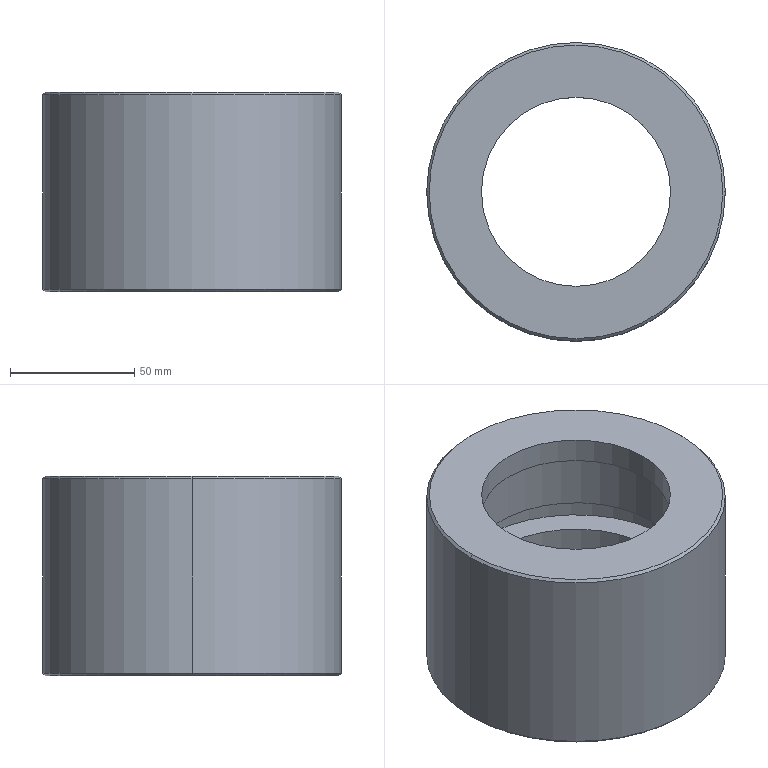Part | SolidWorks | features ICE 4, Chamfer 1, Extrusion 1 | 1 solid | 25 faces | box 120 x 120 x 80 mm | volume 384227 mm3 | cylinder 14 | plane 7 | cone 4 | commonest cylinder face diameters 85 x6 105 x4 76 x2 120 x2
STEP:
#1=CARTESIAN_POINT('',(52.5,0.,46.));
#2=VERTEX_POINT('',#1);
#3=CARTESIAN_POINT('',(-52.5,0.,46.));
#4=VERTEX_POINT('',#3);
#5=CARTESIAN_POINT('',(0.,0.,46.));
#6=DIRECTION('',(0.,0.,-1.));
#7=DIRECTION('',(-1.,0.,0.));
#8=AXIS2_PLACEMENT_3D('',#5,#6,#7);
#9=CIRCLE('',#8,52.5);
#10=EDGE_CURVE('',#2,#4,#9,.T.);
#11=ORIENTED_EDGE('',*,*,#10,.F.);
#12=CARTESIAN_POINT('',(52.5,0.,33.));
#13=VERTEX_POINT('',#12);
#14=CARTESIAN_POINT('',(52.5,0.,46.));
#15=DIRECTION('',(0.,0.,-1.));
#16=VECTOR('',#15,1000.);
#17=LINE('',#14,#16);
#18=EDGE_CURVE('',#2,#13,#17,.T.);
#19=ORIENTED_EDGE('',*,*,#18,.T.);
#20=CARTESIAN_POINT('',(-52.5,0.,33.));
#21=VERTEX_POINT('',#20);
#22=CARTESIAN_POINT('',(0.,0.,33.));
#23=DIRECTION('',(0.,0.,-1.));
#24=DIRECTION('',(-1.,0.,0.));
#25=AXIS2_PLACEMENT_3D('',#22,#23,#24);
#26=CIRCLE('',#25,52.5);
#27=EDGE_CURVE('',#13,#21,#26,.T.);
#28=ORIENTED_EDGE('',*,*,#27,.T.);
#29=CARTESIAN_POINT('',(-52.5,0.,46.));
#30=DIRECTION('',(0.,0.,-1.));
#31=VECTOR('',#30,1000.);
#32=LINE('',#29,#31);
#33=EDGE_CURVE('',#4,#21,#32,.T.);
#34=ORIENTED_EDGE('',*,*,#33,.F.);
#35=EDGE_LOOP('',(#11,#19,#28,#34));
#36=FACE_OUTER_BOUND('',#35,.T.);
#37=CARTESIAN_POINT('',(0.,0.,46.));
#38=DIRECTION('',(0.,0.,-1.));
#39=DIRECTION('',(-1.,0.,0.));
#40=AXIS2_PLACEMENT_3D('',#37,#38,#39);
#41=CYLINDRICAL_SURFACE('',#40,52.5);
#42=ADVANCED_FACE('',(#36),#41,.F.);
#43=CARTESIAN_POINT('',(52.5,0.,23.));
#44=VERTEX_POINT('',#43);
#45=CARTESIAN_POINT('',(-52.5,0.,23.));
#46=VERTEX_POINT('',#45);
#47=CARTESIAN_POINT('',(0.,0.,23.));
#48=DIRECTION('',(0.,0.,-1.));
#49=DIRECTION('',(-1.,0.,0.));
#50=AXIS2_PLACEMENT_3D('',#47,#48,#49);
#51=CIRCLE('',#50,52.5);
#52=EDGE_CURVE('',#44,#46,#51,.T.);
#53=ORIENTED_EDGE('',*,*,#52,.F.);
#54=CARTESIAN_POINT('',(52.5,0.,10.));
#55=VERTEX_POINT('',#54);
#56=CARTESIAN_POINT('',(52.5,0.,23.));
#57=DIRECTION('',(0.,0.,-1.));
#58=VECTOR('',#57,1000.);
#59=LINE('',#56,#58);
#60=EDGE_CURVE('',#44,#55,#59,.T.);
#61=ORIENTED_EDGE('',*,*,#60,.T.);
#62=CARTESIAN_POINT('',(-52.5,0.,10.));
#63=VERTEX_POINT('',#62);
#64=CARTESIAN_POINT('',(0.,0.,10.));
#65=DIRECTION('',(0.,0.,-1.));
#66=DIRECTION('',(-1.,0.,0.));
#67=AXIS2_PLACEMENT_3D('',#64,#65,#66);
#68=CIRCLE('',#67,52.5);
#69=EDGE_CURVE('',#55,#63,#68,.T.);
#70=ORIENTED_EDGE('',*,*,#69,.T.);
#71=CARTESIAN_POINT('',(-52.5,0.,23.));
#72=DIRECTION('',(0.,0.,-1.));
#73=VECTOR('',#72,1000.);
#74=LINE('',#71,#73);
#75=EDGE_CURVE('',#46,#63,#74,.T.);
#76=ORIENTED_EDGE('',*,*,#75,.F.);
#77=EDGE_LOOP('',(#53,#61,#70,#76));
#78=FACE_OUTER_BOUND('',#77,.T.);
#79=CARTESIAN_POINT('',(0.,0.,23.));
#80=DIRECTION('',(0.,0.,-1.));
#81=DIRECTION('',(-1.,0.,0.));
#82=AXIS2_PLACEMENT_3D('',#79,#80,#81);
#83=CYLINDRICAL_SURFACE('',#82,52.5);
#84=ADVANCED_FACE('',(#78),#83,.F.);
#85=CARTESIAN_POINT('',(59.,0.,80.));
#86=VERTEX_POINT('',#85);
#87=CARTESIAN_POINT('',(-59.,0.,80.));
#88=VERTEX_POINT('',#87);
#89=CARTESIAN_POINT('',(0.,0.,80.));
#90=DIRECTION('',(0.,0.,1.));
#91=DIRECTION('',(1.,0.,0.));
#92=AXIS2_PLACEMENT_3D('',#89,#90,#91);
#93=CIRCLE('',#92,59.);
#94=EDGE_CURVE('',#86,#88,#93,.T.);
#95=ORIENTED_EDGE('',*,*,#94,.F.);
#96=CARTESIAN_POINT('',(60.,0.,79.));
#97=VERTEX_POINT('',#96);
#98=CARTESIAN_POINT('',(59.,0.,80.));
#99=DIRECTION('',(0.7071,0.,-0.7071));
#100=VECTOR('',#99,1000.);
#101=LINE('',#98,#100);
#102=EDGE_CURVE('',#86,#97,#101,.T.);
#103=ORIENTED_EDGE('',*,*,#102,.T.);
#104=CARTESIAN_POINT('',(-60.,0.,79.));
#105=VERTEX_POINT('',#104);
#106=CARTESIAN_POINT('',(0.,0.,79.));
#107=DIRECTION('',(0.,0.,-1.));
#108=DIRECTION('',(1.,0.,0.));
#109=AXIS2_PLACEMENT_3D('',#106,#107,#108);
#110=CIRCLE('',#109,60.);
#111=EDGE_CURVE('',#105,#97,#110,.T.);
#112=ORIENTED_EDGE('',*,*,#111,.F.);
#113=CARTESIAN_POINT('',(-59.,0.,80.));
#114=DIRECTION('',(-0.7071,0.,-0.7071));
#115=VECTOR('',#114,1000.);
#116=LINE('',#113,#115);
#117=EDGE_CURVE('',#88,#105,#116,.T.);
#118=ORIENTED_EDGE('',*,*,#117,.F.);
#119=EDGE_LOOP('',(#95,#103,#112,#118));
#120=FACE_OUTER_BOUND('',#119,.T.);
#121=CARTESIAN_POINT('',(0.,0.,80.));
#122=DIRECTION('',(0.,0.,-1.));
#123=DIRECTION('',(-1.,0.,0.));
#124=AXIS2_PLACEMENT_3D('',#121,#122,#123);
#125=CONICAL_SURFACE('',#124,59.,0.7854);
#126=ADVANCED_FACE('',(#120),#125,.T.);
#127=CARTESIAN_POINT('',(-59.,0.,0.));
#128=VERTEX_POINT('',#127);
#129=CARTESIAN_POINT('',(59.,0.,0.));
#130=VERTEX_POINT('',#129);
#131=CARTESIAN_POINT('',(0.,0.,0.));
#132=DIRECTION('',(0.,0.,-1.));
#133=DIRECTION('',(1.,0.,0.));
#134=AXIS2_PLACEMENT_3D('',#131,#132,#133);
#135=CIRCLE('',#134,59.);
#136=EDGE_CURVE('',#128,#130,#135,.T.);
#137=ORIENTED_EDGE('',*,*,#136,.F.);
#138=CARTESIAN_POINT('',(-60.,0.,1.));
#139=VERTEX_POINT('',#138);
#140=CARTESIAN_POINT('',(-60.,0.,1.));
#141=DIRECTION('',(-0.7071,0.,0.7071));
#142=VECTOR('',#141,1000.);
#143=LINE('',#140,#142);
#144=EDGE_CURVE('',#128,#139,#143,.T.);
#145=ORIENTED_EDGE('',*,*,#144,.T.);
#146=CARTESIAN_POINT('',(60.,0.,1.));
#147=VERTEX_POINT('',#146);
#148=CARTESIAN_POINT('',(0.,0.,1.));
#149=DIRECTION('',(0.,0.,1.));
#150=DIRECTION('',(1.,0.,0.));
#151=AXIS2_PLACEMENT_3D('',#148,#149,#150);
#152=CIRCLE('',#151,60.);
#153=EDGE_CURVE('',#147,#139,#152,.T.);
#154=ORIENTED_EDGE('',*,*,#153,.F.);
#155=CARTESIAN_POINT('',(60.,0.,1.));
#156=DIRECTION('',(0.7071,0.,0.7071));
#157=VECTOR('',#156,1000.);
#158=LINE('',#155,#157);
#159=EDGE_CURVE('',#130,#147,#158,.T.);
#160=ORIENTED_EDGE('',*,*,#159,.F.);
#161=EDGE_LOOP('',(#137,#145,#154,#160));
#162=FACE_OUTER_BOUND('',#161,.T.);
#163=CARTESIAN_POINT('',(0.,0.,1.));
#164=DIRECTION('',(0.,0.,1.));
#165=DIRECTION('',(1.,0.,0.));
#166=AXIS2_PLACEMENT_3D('',#163,#164,#165);
#167=CONICAL_SURFACE('',#166,60.,0.7854);
#168=ADVANCED_FACE('',(#162),#167,.T.);
#169=CARTESIAN_POINT('',(38.,0.,70.));
#170=VERTEX_POINT('',#169);
#171=CARTESIAN_POINT('',(-38.,0.,70.));
#172=VERTEX_POINT('',#171);
#173=CARTESIAN_POINT('',(0.,0.,70.));
#174=DIRECTION('',(0.,0.,-1.));
#175=DIRECTION('',(-1.,0.,0.));
#176=AXIS2_PLACEMENT_3D('',#173,#174,#175);
#177=CIRCLE('',#176,38.);
#178=EDGE_CURVE('',#170,#172,#177,.T.);
#179=ORIENTED_EDGE('',*,*,#178,.T.);
#180=CARTESIAN_POINT('',(-38.,0.,80.));
#181=VERTEX_POINT('',#180);
#182=CARTESIAN_POINT('',(-38.,0.,10.));
#183=DIRECTION('',(0.,0.,1.));
#184=VECTOR('',#183,1000.);
#185=LINE('',#182,#184);
#186=EDGE_CURVE('',#172,#181,#185,.T.);
#187=ORIENTED_EDGE('',*,*,#186,.T.);
#188=CARTESIAN_POINT('',(38.,0.,80.));
#189=VERTEX_POINT('',#188);
#190=CARTESIAN_POINT('',(0.,0.,80.));
#191=DIRECTION('',(0.,0.,1.));
#192=DIRECTION('',(1.,0.,0.));
#193=AXIS2_PLACEMENT_3D('',#190,#191,#192);
#194=CIRCLE('',#193,38.);
#195=EDGE_CURVE('',#181,#189,#194,.T.);
#196=ORIENTED_EDGE('',*,*,#195,.T.);
#197=CARTESIAN_POINT('',(38.,0.,10.));
#198=DIRECTION('',(0.,0.,1.));
#199=VECTOR('',#198,1000.);
#200=LINE('',#197,#199);
#201=EDGE_CURVE('',#170,#189,#200,.T.);
#202=ORIENTED_EDGE('',*,*,#201,.F.);
#203=EDGE_LOOP('',(#179,#187,#196,#202));
#204=FACE_OUTER_BOUND('',#203,.T.);
#205=CARTESIAN_POINT('',(0.,0.,10.));
#206=DIRECTION('',(0.,0.,1.));
#207=DIRECTION('',(1.,0.,0.));
#208=AXIS2_PLACEMENT_3D('',#205,#206,#207);
#209=CYLINDRICAL_SURFACE('',#208,38.);
#210=ADVANCED_FACE('',(#204),#209,.F.);
#211=CARTESIAN_POINT('',(42.5,0.,10.));
#212=VERTEX_POINT('',#211);
#213=CARTESIAN_POINT('',(-42.5,0.,10.));
#214=VERTEX_POINT('',#213);
#215=CARTESIAN_POINT('',(0.,0.,10.));
#216=DIRECTION('',(0.,0.,-1.));
#217=DIRECTION('',(-1.,0.,0.));
#218=AXIS2_PLACEMENT_3D('',#215,#216,#217);
#219=CIRCLE('',#218,42.5);
#220=EDGE_CURVE('',#212,#214,#219,.T.);
#221=ORIENTED_EDGE('',*,*,#220,.F.);
#222=CARTESIAN_POINT('',(42.5,0.,0.));
#223=VERTEX_POINT('',#222);
#224=CARTESIAN_POINT('',(42.5,0.,70.));
#225=DIRECTION('',(0.,0.,-1.));
#226=VECTOR('',#225,1000.);
#227=LINE('',#224,#226);
#228=EDGE_CURVE('',#212,#223,#227,.T.);
#229=ORIENTED_EDGE('',*,*,#228,.T.);
#230=CARTESIAN_POINT('',(-42.5,0.,0.));
#231=VERTEX_POINT('',#230);
#232=CARTESIAN_POINT('',(0.,0.,0.));
#233=DIRECTION('',(0.,0.,-1.));
#234=DIRECTION('',(-1.,0.,0.));
#235=AXIS2_PLACEMENT_3D('',#232,#233,#234);
#236=CIRCLE('',#235,42.5);
#237=EDGE_CURVE('',#223,#231,#236,.T.);
#238=ORIENTED_EDGE('',*,*,#237,.T.);
#239=CARTESIAN_POINT('',(-42.5,0.,70.));
#240=DIRECTION('',(0.,0.,-1.));
#241=VECTOR('',#240,1000.);
#242=LINE('',#239,#241);
#243=EDGE_CURVE('',#214,#231,#242,.T.);
#244=ORIENTED_EDGE('',*,*,#243,.F.);
#245=EDGE_LOOP('',(#221,#229,#238,#244));
#246=FACE_OUTER_BOUND('',#245,.T.);
#247=CARTESIAN_POINT('',(0.,0.,70.));
#248=DIRECTION('',(0.,0.,-1.));
#249=DIRECTION('',(-1.,0.,0.));
#250=AXIS2_PLACEMENT_3D('',#247,#248,#249);
#251=CYLINDRICAL_SURFACE('',#250,42.5);
#252=ADVANCED_FACE('',(#246),#251,.F.);
#253=ORIENTED_EDGE('',*,*,#111,.T.);
#254=CARTESIAN_POINT('',(60.,0.,80.));
#255=DIRECTION('',(0.,0.,-1.));
#256=VECTOR('',#255,1000.);
#257=LINE('',#254,#256);
#258=EDGE_CURVE('',#97,#147,#257,.T.);
#259=ORIENTED_EDGE('',*,*,#258,.T.);
#260=ORIENTED_EDGE('',*,*,#153,.T.);
#261=CARTESIAN_POINT('',(-60.,0.,80.));
#262=DIRECTION('',(0.,0.,-1.));
#263=VECTOR('',#262,1000.);
#264=LINE('',#261,#263);
#265=EDGE_CURVE('',#105,#139,#264,.T.);
#266=ORIENTED_EDGE('',*,*,#265,.F.);
#267=EDGE_LOOP('',(#253,#259,#260,#266));
#268=FACE_OUTER_BOUND('',#267,.T.);
#269=CARTESIAN_POINT('',(0.,0.,80.));
#270=DIRECTION('',(0.,0.,-1.));
#271=DIRECTION('',(-1.,0.,0.));
#272=AXIS2_PLACEMENT_3D('',#269,#270,#271);
#273=CYLINDRICAL_SURFACE('',#272,60.);
#274=ADVANCED_FACE('',(#268),#273,.T.);
#275=CARTESIAN_POINT('',(42.5,0.,33.));
#276=VERTEX_POINT('',#275);
#277=CARTESIAN_POINT('',(-42.5,0.,33.));
#278=VERTEX_POINT('',#277);
#279=CARTESIAN_POINT('',(0.,0.,33.));
#280=DIRECTION('',(0.,0.,-1.));
#281=DIRECTION('',(-1.,0.,0.));
#282=AXIS2_PLACEMENT_3D('',#279,#280,#281);
#283=CIRCLE('',#282,42.5);
#284=EDGE_CURVE('',#276,#278,#283,.T.);
#285=ORIENTED_EDGE('',*,*,#284,.F.);
#286=CARTESIAN_POINT('',(42.5,0.,23.));
#287=VERTEX_POINT('',#286);
#288=CARTESIAN_POINT('',(42.5,0.,70.));
#289=DIRECTION('',(0.,0.,-1.));
#290=VECTOR('',#289,1000.);
#291=LINE('',#288,#290);
#292=EDGE_CURVE('',#276,#287,#291,.T.);
#293=ORIENTED_EDGE('',*,*,#292,.T.);
#294=CARTESIAN_POINT('',(-42.5,0.,23.));
#295=VERTEX_POINT('',#294);
#296=CARTESIAN_POINT('',(0.,0.,23.));
#297=DIRECTION('',(0.,0.,-1.));
#298=DIRECTION('',(-1.,0.,0.));
#299=AXIS2_PLACEMENT_3D('',#296,#297,#298);
#300=CIRCLE('',#299,42.5);
#301=EDGE_CURVE('',#287,#295,#300,.T.);
#302=ORIENTED_EDGE('',*,*,#301,.T.);
#303=CARTESIAN_POINT('',(-42.5,0.,70.));
#304=DIRECTION('',(0.,0.,-1.));
#305=VECTOR('',#304,1000.);
#306=LINE('',#303,#305);
#307=EDGE_CURVE('',#278,#295,#306,.T.);
#308=ORIENTED_EDGE('',*,*,#307,.F.);
#309=EDGE_LOOP('',(#285,#293,#302,#308));
#310=FACE_OUTER_BOUND('',#309,.T.);
#311=CARTESIAN_POINT('',(0.,0.,70.));
#312=DIRECTION('',(0.,0.,-1.));
#313=DIRECTION('',(-1.,0.,0.));
#314=AXIS2_PLACEMENT_3D('',#311,#312,#313);
#315=CYLINDRICAL_SURFACE('',#314,42.5);
#316=ADVANCED_FACE('',(#310),#315,.F.);
#317=CARTESIAN_POINT('',(42.5,0.,70.));
#318=VERTEX_POINT('',#317);
#319=CARTESIAN_POINT('',(-42.5,0.,70.));
#320=VERTEX_POINT('',#319);
#321=CARTESIAN_POINT('',(0.,0.,70.));
#322=DIRECTION('',(0.,0.,-1.));
#323=DIRECTION('',(-1.,0.,0.));
#324=AXIS2_PLACEMENT_3D('',#321,#322,#323);
#325=CIRCLE('',#324,42.5);
#326=EDGE_CURVE('',#318,#320,#325,.T.);
#327=ORIENTED_EDGE('',*,*,#326,.F.);
#328=CARTESIAN_POINT('',(42.5,0.,46.));
#329=VERTEX_POINT('',#328);
#330=CARTESIAN_POINT('',(42.5,0.,70.));
#331=DIRECTION('',(0.,0.,-1.));
#332=VECTOR('',#331,1000.);
#333=LINE('',#330,#332);
#334=EDGE_CURVE('',#318,#329,#333,.T.);
#335=ORIENTED_EDGE('',*,*,#334,.T.);
#336=CARTESIAN_POINT('',(-42.5,0.,46.));
#337=VERTEX_POINT('',#336);
#338=CARTESIAN_POINT('',(0.,0.,46.));
#339=DIRECTION('',(0.,0.,-1.));
#340=DIRECTION('',(-1.,0.,0.));
#341=AXIS2_PLACEMENT_3D('',#338,#339,#340);
#342=CIRCLE('',#341,42.5);
#343=EDGE_CURVE('',#329,#337,#342,.T.);
#344=ORIENTED_EDGE('',*,*,#343,.T.);
#345=CARTESIAN_POINT('',(-42.5,0.,70.));
#346=DIRECTION('',(0.,0.,-1.));
#347=VECTOR('',#346,1000.);
#348=LINE('',#345,#347);
#349=EDGE_CURVE('',#320,#337,#348,.T.);
#350=ORIENTED_EDGE('',*,*,#349,.F.);
#351=EDGE_LOOP('',(#327,#335,#344,#350));
#352=FACE_OUTER_BOUND('',#351,.T.);
#353=CARTESIAN_POINT('',(0.,0.,70.));
#354=DIRECTION('',(0.,0.,-1.));
#355=DIRECTION('',(-1.,0.,0.));
#356=AXIS2_PLACEMENT_3D('',#353,#354,#355);
#357=CYLINDRICAL_SURFACE('',#356,42.5);
#358=ADVANCED_FACE('',(#352),#357,.F.);
#359=ORIENTED_EDGE('',*,*,#334,.F.);
#360=CARTESIAN_POINT('',(0.,0.,70.));
#361=DIRECTION('',(0.,0.,-1.));
#362=DIRECTION('',(-1.,0.,0.));
#363=AXIS2_PLACEMENT_3D('',#360,#361,#362);
#364=CIRCLE('',#363,42.5);
#365=EDGE_CURVE('',#320,#318,#364,.T.);
#366=ORIENTED_EDGE('',*,*,#365,.F.);
#367=ORIENTED_EDGE('',*,*,#349,.T.);
#368=CARTESIAN_POINT('',(0.,0.,46.));
#369=DIRECTION('',(0.,0.,-1.));
#370=DIRECTION('',(-1.,0.,0.));
#371=AXIS2_PLACEMENT_3D('',#368,#369,#370);
#372=CIRCLE('',#371,42.5);
#373=EDGE_CURVE('',#337,#329,#372,.T.);
#374=ORIENTED_EDGE('',*,*,#373,.T.);
#375=EDGE_LOOP('',(#359,#366,#367,#374));
#376=FACE_OUTER_BOUND('',#375,.T.);
#377=CARTESIAN_POINT('',(0.,0.,70.));
#378=DIRECTION('',(0.,0.,-1.));
#379=DIRECTION('',(-1.,0.,0.));
#380=AXIS2_PLACEMENT_3D('',#377,#378,#379);
#381=CYLINDRICAL_SURFACE('',#380,42.5);
#382=ADVANCED_FACE('',(#376),#381,.F.);
#383=ORIENTED_EDGE('',*,*,#292,.F.);
#384=CARTESIAN_POINT('',(0.,0.,33.));
#385=DIRECTION('',(0.,0.,-1.));
#386=DIRECTION('',(-1.,0.,0.));
#387=AXIS2_PLACEMENT_3D('',#384,#385,#386);
#388=CIRCLE('',#387,42.5);
#389=EDGE_CURVE('',#278,#276,#388,.T.);
#390=ORIENTED_EDGE('',*,*,#389,.F.);
#391=ORIENTED_EDGE('',*,*,#307,.T.);
#392=CARTESIAN_POINT('',(0.,0.,23.));
#393=DIRECTION('',(0.,0.,-1.));
#394=DIRECTION('',(-1.,0.,0.));
#395=AXIS2_PLACEMENT_3D('',#392,#393,#394);
#396=CIRCLE('',#395,42.5);
#397=EDGE_CURVE('',#295,#287,#396,.T.);
#398=ORIENTED_EDGE('',*,*,#397,.T.);
#399=EDGE_LOOP('',(#383,#390,#391,#398));
#400=FACE_OUTER_BOUND('',#399,.T.);
#401=CARTESIAN_POINT('',(0.,0.,70.));
#402=DIRECTION('',(0.,0.,-1.));
#403=DIRECTION('',(-1.,0.,0.));
#404=AXIS2_PLACEMENT_3D('',#401,#402,#403);
#405=CYLINDRICAL_SURFACE('',#404,42.5);
#406=ADVANCED_FACE('',(#400),#405,.F.);
#407=ORIENTED_EDGE('',*,*,#258,.F.);
#408=CARTESIAN_POINT('',(0.,0.,79.));
#409=DIRECTION('',(0.,0.,-1.));
#410=DIRECTION('',(1.,0.,0.));
#411=AXIS2_PLACEMENT_3D('',#408,#409,#410);
#412=CIRCLE('',#411,60.);
#413=EDGE_CURVE('',#97,#105,#412,.T.);
#414=ORIENTED_EDGE('',*,*,#413,.T.);
#415=ORIENTED_EDGE('',*,*,#265,.T.);
#416=CARTESIAN_POINT('',(0.,0.,1.));
#417=DIRECTION('',(0.,0.,1.));
#418=DIRECTION('',(1.,0.,0.));
#419=AXIS2_PLACEMENT_3D('',#416,#417,#418);
#420=CIRCLE('',#419,60.);
#421=EDGE_CURVE('',#139,#147,#420,.T.);
#422=ORIENTED_EDGE('',*,*,#421,.T.);
#423=EDGE_LOOP('',(#407,#414,#415,#422));
#424=FACE_OUTER_BOUND('',#423,.T.);
#425=CARTESIAN_POINT('',(0.,0.,80.));
#426=DIRECTION('',(0.,0.,-1.));
#427=DIRECTION('',(-1.,0.,0.));
#428=AXIS2_PLACEMENT_3D('',#425,#426,#427);
#429=CYLINDRICAL_SURFACE('',#428,60.);
#430=ADVANCED_FACE('',(#424),#429,.T.);
#431=CARTESIAN_POINT('',(0.,0.,80.));
#432=DIRECTION('',(0.,0.,1.));
#433=DIRECTION('',(1.,0.,0.));
#434=AXIS2_PLACEMENT_3D('',#431,#432,#433);
#435=CIRCLE('',#434,59.);
#436=EDGE_CURVE('',#88,#86,#435,.T.);
#437=ORIENTED_EDGE('',*,*,#436,.T.);
#438=ORIENTED_EDGE('',*,*,#94,.T.);
#439=EDGE_LOOP('',(#437,#438));
#440=FACE_OUTER_BOUND('',#439,.T.);
#441=CARTESIAN_POINT('',(0.,0.,80.));
#442=DIRECTION('',(0.,0.,1.));
#443=DIRECTION('',(1.,0.,0.));
#444=AXIS2_PLACEMENT_3D('',#441,#442,#443);
#445=CIRCLE('',#444,38.);
#446=EDGE_CURVE('',#189,#181,#445,.T.);
#447=ORIENTED_EDGE('',*,*,#446,.F.);
#448=ORIENTED_EDGE('',*,*,#195,.F.);
#449=EDGE_LOOP('',(#447,#448));
#450=FACE_BOUND('',#449,.T.);
#451=CARTESIAN_POINT('',(0.,0.,80.));
#452=DIRECTION('',(0.,0.,1.));
#453=DIRECTION('',(1.,0.,0.));
#454=AXIS2_PLACEMENT_3D('',#451,#452,#453);
#455=PLANE('',#454);
#456=ADVANCED_FACE('',(#440,#450),#455,.T.);
#457=CARTESIAN_POINT('',(0.,0.,0.));
#458=DIRECTION('',(0.,0.,-1.));
#459=DIRECTION('',(1.,0.,0.));
#460=AXIS2_PLACEMENT_3D('',#457,#458,#459);
#461=CIRCLE('',#460,59.);
#462=EDGE_CURVE('',#130,#128,#461,.T.);
#463=ORIENTED_EDGE('',*,*,#462,.T.);
#464=ORIENTED_EDGE('',*,*,#136,.T.);
#465=EDGE_LOOP('',(#463,#464));
#466=FACE_OUTER_BOUND('',#465,.T.);
#467=CARTESIAN_POINT('',(0.,0.,0.));
#468=DIRECTION('',(0.,0.,-1.));
#469=DIRECTION('',(-1.,0.,0.));
#470=AXIS2_PLACEMENT_3D('',#467,#468,#469);
#471=CIRCLE('',#470,42.5);
#472=EDGE_CURVE('',#231,#223,#471,.T.);
#473=ORIENTED_EDGE('',*,*,#472,.F.);
#474=ORIENTED_EDGE('',*,*,#237,.F.);
#475=EDGE_LOOP('',(#473,#474));
#476=FACE_BOUND('',#475,.T.);
#477=CARTESIAN_POINT('',(0.,0.,0.));
#478=DIRECTION('',(0.,0.,1.));
#479=DIRECTION('',(1.,0.,0.));
#480=AXIS2_PLACEMENT_3D('',#477,#478,#479);
#481=PLANE('',#480);
#482=ADVANCED_FACE('',(#466,#476),#481,.F.);
#483=ORIENTED_EDGE('',*,*,#228,.F.);
#484=CARTESIAN_POINT('',(0.,0.,10.));
#485=DIRECTION('',(0.,0.,-1.));
#486=DIRECTION('',(-1.,0.,0.));
#487=AXIS2_PLACEMENT_3D('',#484,#485,#486);
#488=CIRCLE('',#487,42.5);
#489=EDGE_CURVE('',#214,#212,#488,.T.);
#490=ORIENTED_EDGE('',*,*,#489,.F.);
#491=ORIENTED_EDGE('',*,*,#243,.T.);
#492=ORIENTED_EDGE('',*,*,#472,.T.);
#493=EDGE_LOOP('',(#483,#490,#491,#492));
#494=FACE_OUTER_BOUND('',#493,.T.);
#495=CARTESIAN_POINT('',(0.,0.,70.));
#496=DIRECTION('',(0.,0.,-1.));
#497=DIRECTION('',(-1.,0.,0.));
#498=AXIS2_PLACEMENT_3D('',#495,#496,#497);
#499=CYLINDRICAL_SURFACE('',#498,42.5);
#500=ADVANCED_FACE('',(#494),#499,.F.);
#501=ORIENTED_EDGE('',*,*,#178,.F.);
#502=CARTESIAN_POINT('',(0.,0.,70.));
#503=DIRECTION('',(0.,0.,-1.));
#504=DIRECTION('',(-1.,0.,0.));
#505=AXIS2_PLACEMENT_3D('',#502,#503,#504);
#506=CIRCLE('',#505,38.);
#507=EDGE_CURVE('',#172,#170,#506,.T.);
#508=ORIENTED_EDGE('',*,*,#507,.F.);
#509=EDGE_LOOP('',(#501,#508));
#510=FACE_BOUND('',#509,.T.);
#511=ORIENTED_EDGE('',*,*,#365,.T.);
#512=ORIENTED_EDGE('',*,*,#326,.T.);
#513=EDGE_LOOP('',(#511,#512));
#514=FACE_OUTER_BOUND('',#513,.T.);
#515=CARTESIAN_POINT('',(0.,0.,70.));
#516=DIRECTION('',(0.,0.,-1.));
#517=DIRECTION('',(-1.,0.,0.));
#518=AXIS2_PLACEMENT_3D('',#515,#516,#517);
#519=PLANE('',#518);
#520=ADVANCED_FACE('',(#510,#514),#519,.T.);
#521=ORIENTED_EDGE('',*,*,#186,.F.);
#522=ORIENTED_EDGE('',*,*,#507,.T.);
#523=ORIENTED_EDGE('',*,*,#201,.T.);
#524=ORIENTED_EDGE('',*,*,#446,.T.);
#525=EDGE_LOOP('',(#521,#522,#523,#524));
#526=FACE_OUTER_BOUND('',#525,.T.);
#527=CARTESIAN_POINT('',(0.,0.,10.));
#528=DIRECTION('',(0.,0.,1.));
#529=DIRECTION('',(1.,0.,0.));
#530=AXIS2_PLACEMENT_3D('',#527,#528,#529);
#531=CYLINDRICAL_SURFACE('',#530,38.);
#532=ADVANCED_FACE('',(#526),#531,.F.);
#533=ORIENTED_EDGE('',*,*,#144,.F.);
#534=ORIENTED_EDGE('',*,*,#462,.F.);
#535=ORIENTED_EDGE('',*,*,#159,.T.);
#536=ORIENTED_EDGE('',*,*,#421,.F.);
#537=EDGE_LOOP('',(#533,#534,#535,#536));
#538=FACE_OUTER_BOUND('',#537,.T.);
#539=CARTESIAN_POINT('',(0.,0.,1.));
#540=DIRECTION('',(0.,0.,1.));
#541=DIRECTION('',(1.,0.,0.));
#542=AXIS2_PLACEMENT_3D('',#539,#540,#541);
#543=CONICAL_SURFACE('',#542,60.,0.7854);
#544=ADVANCED_FACE('',(#538),#543,.T.);
#545=ORIENTED_EDGE('',*,*,#102,.F.);
#546=ORIENTED_EDGE('',*,*,#436,.F.);
#547=ORIENTED_EDGE('',*,*,#117,.T.);
#548=ORIENTED_EDGE('',*,*,#413,.F.);
#549=EDGE_LOOP('',(#545,#546,#547,#548));
#550=FACE_OUTER_BOUND('',#549,.T.);
#551=CARTESIAN_POINT('',(0.,0.,80.));
#552=DIRECTION('',(0.,0.,-1.));
#553=DIRECTION('',(-1.,0.,0.));
#554=AXIS2_PLACEMENT_3D('',#551,#552,#553);
#555=CONICAL_SURFACE('',#554,59.,0.7854);
#556=ADVANCED_FACE('',(#550),#555,.T.);
#557=ORIENTED_EDGE('',*,*,#60,.F.);
#558=CARTESIAN_POINT('',(0.,0.,23.));
#559=DIRECTION('',(0.,0.,-1.));
#560=DIRECTION('',(-1.,0.,0.));
#561=AXIS2_PLACEMENT_3D('',#558,#559,#560);
#562=CIRCLE('',#561,52.5);
#563=EDGE_CURVE('',#46,#44,#562,.T.);
#564=ORIENTED_EDGE('',*,*,#563,.F.);
#565=ORIENTED_EDGE('',*,*,#75,.T.);
#566=CARTESIAN_POINT('',(0.,0.,10.));
#567=DIRECTION('',(0.,0.,-1.));
#568=DIRECTION('',(-1.,0.,0.));
#569=AXIS2_PLACEMENT_3D('',#566,#567,#568);
#570=CIRCLE('',#569,52.5);
#571=EDGE_CURVE('',#63,#55,#570,.T.);
#572=ORIENTED_EDGE('',*,*,#571,.T.);
#573=EDGE_LOOP('',(#557,#564,#565,#572));
#574=FACE_OUTER_BOUND('',#573,.T.);
#575=CARTESIAN_POINT('',(0.,0.,23.));
#576=DIRECTION('',(0.,0.,-1.));
#577=DIRECTION('',(-1.,0.,0.));
#578=AXIS2_PLACEMENT_3D('',#575,#576,#577);
#579=CYLINDRICAL_SURFACE('',#578,52.5);
#580=ADVANCED_FACE('',(#574),#579,.F.);
#581=ORIENTED_EDGE('',*,*,#397,.F.);
#582=ORIENTED_EDGE('',*,*,#301,.F.);
#583=EDGE_LOOP('',(#581,#582));
#584=FACE_BOUND('',#583,.T.);
#585=ORIENTED_EDGE('',*,*,#563,.T.);
#586=ORIENTED_EDGE('',*,*,#52,.T.);
#587=EDGE_LOOP('',(#585,#586));
#588=FACE_OUTER_BOUND('',#587,.T.);
#589=CARTESIAN_POINT('',(0.,0.,23.));
#590=DIRECTION('',(0.,0.,-1.));
#591=DIRECTION('',(-1.,0.,0.));
#592=AXIS2_PLACEMENT_3D('',#589,#590,#591);
#593=PLANE('',#592);
#594=ADVANCED_FACE('',(#584,#588),#593,.T.);
#595=ORIENTED_EDGE('',*,*,#489,.T.);
#596=ORIENTED_EDGE('',*,*,#220,.T.);
#597=EDGE_LOOP('',(#595,#596));
#598=FACE_BOUND('',#597,.T.);
#599=ORIENTED_EDGE('',*,*,#571,.F.);
#600=ORIENTED_EDGE('',*,*,#69,.F.);
#601=EDGE_LOOP('',(#599,#600));
#602=FACE_OUTER_BOUND('',#601,.T.);
#603=CARTESIAN_POINT('',(0.,0.,10.));
#604=DIRECTION('',(0.,0.,-1.));
#605=DIRECTION('',(-1.,0.,0.));
#606=AXIS2_PLACEMENT_3D('',#603,#604,#605);
#607=PLANE('',#606);
#608=ADVANCED_FACE('',(#598,#602),#607,.F.);
#609=ORIENTED_EDGE('',*,*,#18,.F.);
#610=CARTESIAN_POINT('',(0.,0.,46.));
#611=DIRECTION('',(0.,0.,-1.));
#612=DIRECTION('',(-1.,0.,0.));
#613=AXIS2_PLACEMENT_3D('',#610,#611,#612);
#614=CIRCLE('',#613,52.5);
#615=EDGE_CURVE('',#4,#2,#614,.T.);
#616=ORIENTED_EDGE('',*,*,#615,.F.);
#617=ORIENTED_EDGE('',*,*,#33,.T.);
#618=CARTESIAN_POINT('',(0.,0.,33.));
#619=DIRECTION('',(0.,0.,-1.));
#620=DIRECTION('',(-1.,0.,0.));
#621=AXIS2_PLACEMENT_3D('',#618,#619,#620);
#622=CIRCLE('',#621,52.5);
#623=EDGE_CURVE('',#21,#13,#622,.T.);
#624=ORIENTED_EDGE('',*,*,#623,.T.);
#625=EDGE_LOOP('',(#609,#616,#617,#624));
#626=FACE_OUTER_BOUND('',#625,.T.);
#627=CARTESIAN_POINT('',(0.,0.,46.));
#628=DIRECTION('',(0.,0.,-1.));
#629=DIRECTION('',(-1.,0.,0.));
#630=AXIS2_PLACEMENT_3D('',#627,#628,#629);
#631=CYLINDRICAL_SURFACE('',#630,52.5);
#632=ADVANCED_FACE('',(#626),#631,.F.);
#633=ORIENTED_EDGE('',*,*,#373,.F.);
#634=ORIENTED_EDGE('',*,*,#343,.F.);
#635=EDGE_LOOP('',(#633,#634));
#636=FACE_BOUND('',#635,.T.);
#637=ORIENTED_EDGE('',*,*,#615,.T.);
#638=ORIENTED_EDGE('',*,*,#10,.T.);
#639=EDGE_LOOP('',(#637,#638));
#640=FACE_OUTER_BOUND('',#639,.T.);
#641=CARTESIAN_POINT('',(0.,0.,46.));
#642=DIRECTION('',(0.,0.,-1.));
#643=DIRECTION('',(-1.,0.,0.));
#644=AXIS2_PLACEMENT_3D('',#641,#642,#643);
#645=PLANE('',#644);
#646=ADVANCED_FACE('',(#636,#640),#645,.T.);
#647=ORIENTED_EDGE('',*,*,#389,.T.);
#648=ORIENTED_EDGE('',*,*,#284,.T.);
#649=EDGE_LOOP('',(#647,#648));
#650=FACE_BOUND('',#649,.T.);
#651=ORIENTED_EDGE('',*,*,#623,.F.);
#652=ORIENTED_EDGE('',*,*,#27,.F.);
#653=EDGE_LOOP('',(#651,#652));
#654=FACE_OUTER_BOUND('',#653,.T.);
#655=CARTESIAN_POINT('',(0.,0.,33.));
#656=DIRECTION('',(0.,0.,-1.));
#657=DIRECTION('',(-1.,0.,0.));
#658=AXIS2_PLACEMENT_3D('',#655,#656,#657);
#659=PLANE('',#658);
#660=ADVANCED_FACE('',(#650,#654),#659,.F.);
#661=CLOSED_SHELL('',(#42,#84,#126,#168,#210,#252,#274,#316,#358,#382,#406,#430,#456,#482,#500,#520,#532,#544,#556,#580,#594,#608,#632,#646,#660));
#662=MANIFOLD_SOLID_BREP('',#661);
#663=CARTESIAN_POINT('',(0.,0.,0.));
#664=DIRECTION('',(0.,0.,1.));
#665=DIRECTION('',(1.,0.,0.));
#666=AXIS2_PLACEMENT_3D('',#663,#664,#665);
#667=(LENGTH_UNIT()NAMED_UNIT(*)SI_UNIT(.MILLI.,.METRE.));
#668=UNCERTAINTY_MEASURE_WITH_UNIT(LENGTH_MEASURE(0.00001),#667,'','');
#669=(NAMED_UNIT(*)PLANE_ANGLE_UNIT()SI_UNIT($,.RADIAN.));
#670=(NAMED_UNIT(*)SI_UNIT($,.STERADIAN.)SOLID_ANGLE_UNIT());
#671=(GEOMETRIC_REPRESENTATION_CONTEXT(3)GLOBAL_UNCERTAINTY_ASSIGNED_CONTEXT((#668))GLOBAL_UNIT_ASSIGNED_CONTEXT((#667,#669,#670))REPRESENTATION_CONTEXT('',''));
#672=ADVANCED_BREP_SHAPE_REPRESENTATION('',(#662,#666),#671);